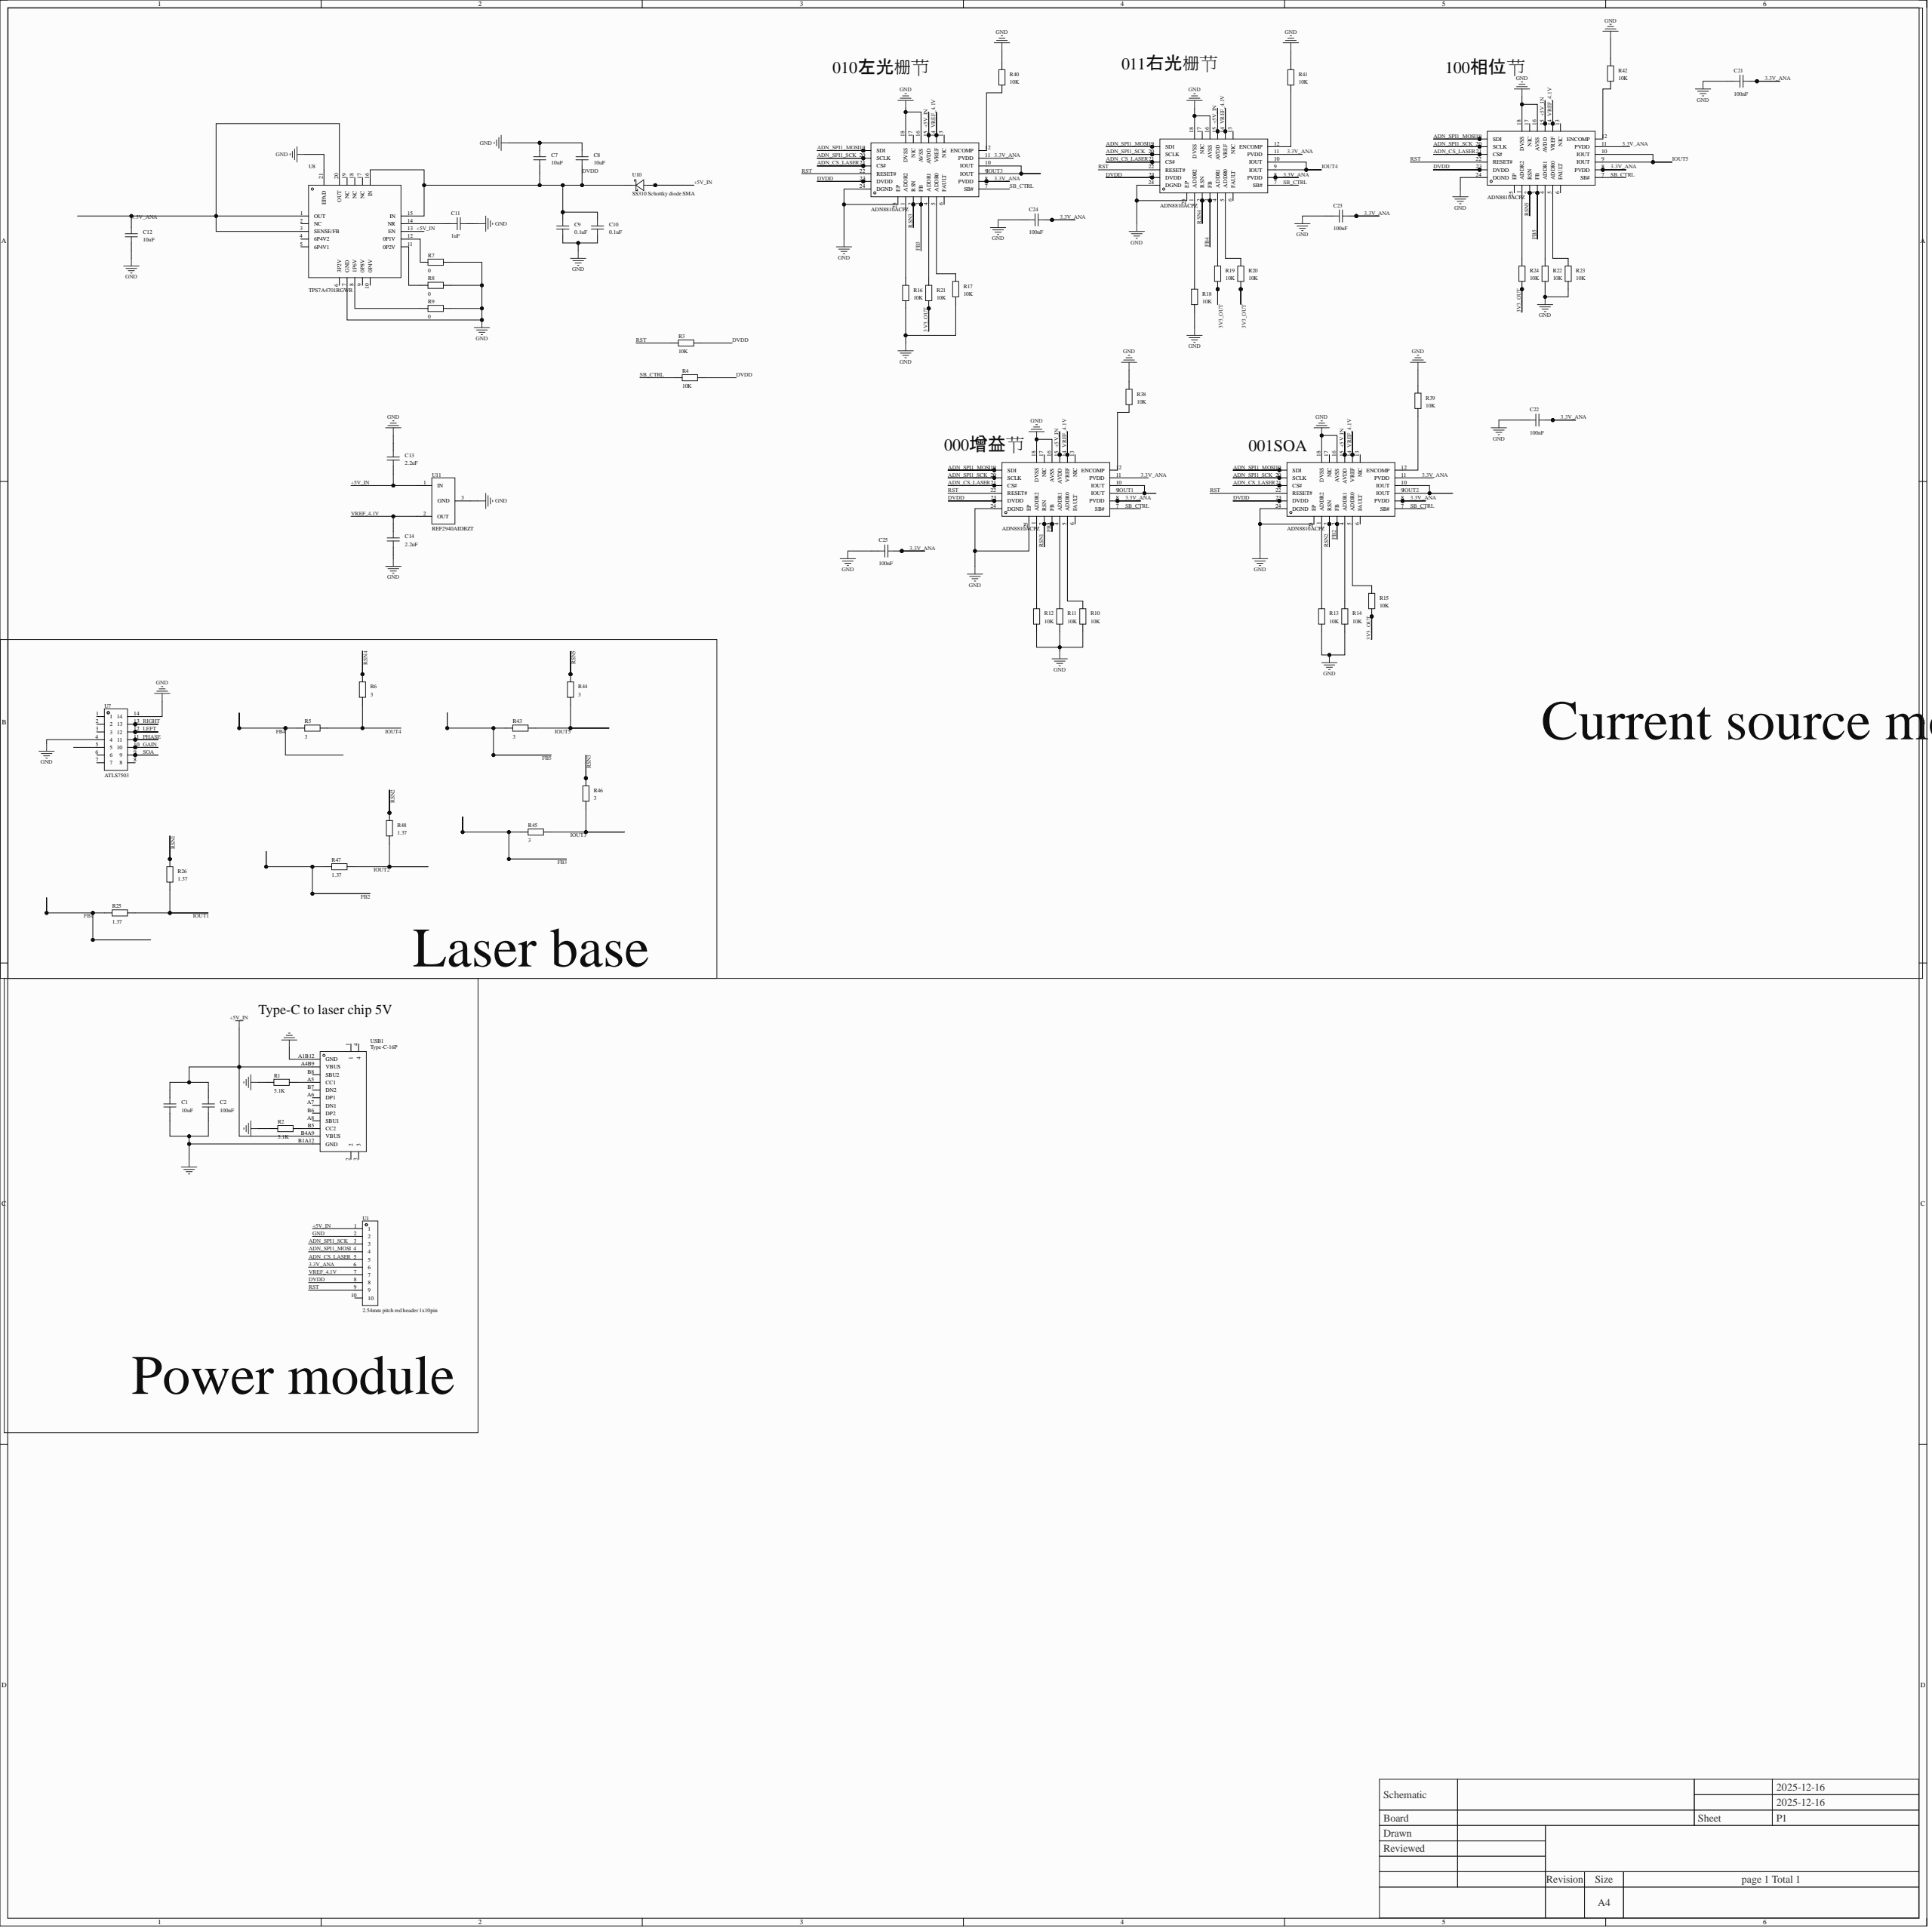Circuit board | Altium Designer | 63 parts | 52 nets
Bill of materials:
Comment,Description,Designator,Footprint,LibRef,Quantity
"ADN8810ACPZ","Output current: 300mA;","000增益节, 001SOA, 010左光栅节, 011右光栅节, 100相位节","LFCSP-24_L4.0-W4.0-P0.50-BL-EP2.3","ADN8810ACPZ","5"
"10uF","Capacitance: 10nF; accuracy: ±10%; rated voltage: 16V; temperature coefficient: X7R;","C1","C0402","AC0402KRX7R7BB103","1"
"100nF","Capacitance: 10nF; accuracy: ±10%; rated voltage: 16V; temperature coefficient: X7R;","C2","C0402","AC0402KRX7R7BB103","1"
"10uF","","C7, C8, C12","C0603","CAP_0603","3"
"0.1uF","","C9, C10","C0603","CAP_0603","2"
"1uF","","C11","C0603","CAP_0603","1"
"2.2uF","","C13, C14","C0603","CAP_0603","2"
"100nF","","C21, C22, C23, C24, C25","C0603","CAP_0603","5"
"5.1K","","R1, R2","R0603","Res_0603","2"
"10K","","R3, R4, R10, R11, R12, R13, R14, R15, R16, R17, R18, R19, R20, R21, R22, R23, R24, R38, R39, R40, R41, R42","R0603","Res_0603","22"
"3","","R5, R6, R43, R44, R45, R46","R0603","Res_0603","6"
"0","","R7, R8, R9","R0603","Res_0603","3"
"1.37","","R25, R26, R47, R48","R0603","Res_0603","4"
"2.54mm pitch red header 1x10pin","","U1","HDR-TH_10P-P2.54-V-F-2","间距2.54mm红色排母座1x10pin","1"
"ATLS7503","","U7","HDR-SMD_14P-P1.27-V-F-R2-C7-LS4.8","HEADER7X2B","1"
"TPS7A4701RGWR","Output type: adjustable; working voltage: 35V; output voltage: 1.4V~34V; output current: 1A; power supply rejection ratio (PSRR): 78dB@(1kHz); output polarity: positive;","U8","VQFN-20_L5.0-W5.0-P0.65-TL-EP","TPS7A4701RGWR","1"
"SS310 Schottky diode SMA","","U10","SMA_L4.3-W2.6-LS5.1-R-RD","SS310肖特基二极管SMA","1"
"REF2940AIDBZT","Output type: fixed; input voltage: 4.146V~5.5V; output voltage: 4.096V; output current: 25mA; accuracy: ±2%;","U11","SOT-23-3_L2.9-W1.3-P1.90-LS2.4-BR","REF2940AIDBZT","1"
"Type-C-16P","","USB1","USB-C-SMD_GT-USB-7010E","Type-C-16P","1"
Netlist (Protel format):
[
000增益节
LFCSP-24_L4.0-W4.0-P0.50-BL-EP2.3
ADN8810ACPZ



]
[
001SOA
LFCSP-24_L4.0-W4.0-P0.50-BL-EP2.3
ADN8810ACPZ



]
[
010左光栅节
LFCSP-24_L4.0-W4.0-P0.50-BL-EP2.3
ADN8810ACPZ



]
[
011右光栅节
LFCSP-24_L4.0-W4.0-P0.50-BL-EP2.3
ADN8810ACPZ



]
[
100相位节
LFCSP-24_L4.0-W4.0-P0.50-BL-EP2.3
ADN8810ACPZ



]
[
C1
C0402
10uF



]
[
C2
C0402
100nF



]
[
C7
C0603
10uF



]
[
C8
C0603
10uF



]
[
C9
C0603
0.1uF



]
[
C10
C0603
0.1uF



]
[
C11
C0603
1uF



]
[
C12
C0603
10uF



]
[
C13
C0603
2.2uF



]
[
C14
C0603
2.2uF



]
[
C21
C0603
100nF



]
[
C22
C0603
100nF



]
[
C23
C0603
100nF



]
[
C24
C0603
100nF



]
[
C25
C0603
100nF



]
[
R1
R0603
5.1K



]
[
R2
R0603
5.1K



]
[
R3
R0603
10K



]
[
R4
R0603
10K



]
[
R5
R0603
3



]
[
R6
R0603
3



]
[
R7
R0603
0



]
[
R8
R0603
0



]
[
R9
R0603
0



]
[
R10
R0603
10K



]
[
R11
R0603
10K



]
[
R12
R0603
10K



]
[
R13
R0603
10K



]
[
R14
R0603
10K



]
[
R15
R0603
10K



]
[
R16
R0603
10K



]
[
R17
R0603
10K



]
[
R18
R0603
10K



]
[
R19
R0603
10K



]
[
R20
R0603
10K



]
[
R21
R0603
10K



]
[
R22
R0603
10K



]
[
R23
R0603
10K



]
[
R24
R0603
10K



]
[
R25
R0603
1.37



]
[
R26
R0603
1.37



]
[
R38
R0603
10K



]
[
R39
R0603
10K



]
[
R40
R0603
10K



]
[
R41
R0603
10K



]
[
R42
R0603
10K



]
[
R43
R0603
3



]
[
R44
R0603
3



]
[
R45
R0603
3



]
[
R46
R0603
3



]
[
R47
R0603
1.37



]
[
R48
R0603
1.37



]
[
U1
HDR-TH_10P-P2.54-V-F-2
2.54mm pitch red header 1x10pin



]
[
U7
HDR-SMD_14P-P1.27-V-F-R2-C7-LS4.8
ATLS7503



]
[
U8
VQFN-20_L5.0-W5.0-P0.65-TL-EP
TPS7A4701RGWR



]
[
U10
SMA_L4.3-W2.6-LS5.1-R-RD
SS310 Schottky diode SMA



]
[
U11
SOT-23-3_L2.9-W1.3-P1.90-LS2.4-BR
REF2940AIDBZT



]
[
USB1
USB-C-SMD_GT-USB-7010E
Type-C-16P



]
(
VREF_4.1V
000增益节-14
001SOA-14
010左光栅节-14
011右光栅节-14
100相位节-14
C14-2
U1-7
U11-2
)
(
SB_CTRL
000增益节-7
001SOA-7
010左光栅节-7
011右光栅节-7
100相位节-7
R4-1
)
(
RST
000增益节-22
001SOA-22
010左光栅节-22
011右光栅节-22
100相位节-22
R3-1
U1-9
)
(
RSN5
100相位节-2
R44-1
)
(
RSN4
011右光栅节-2
R6-1
)
(
RSN3
010左光栅节-2
R46-1
)
(
RSN2
001SOA-2
R48-1
)
(
RSN1
000增益节-2
R26-1
)
(
NetR9_1
R9-1
U8-8
)
(
NetR8_1
R8-1
U8-11
)
(
NetR7_1
R7-1
U8-12
)
(
NetR2_2
R2-2
USB1-B5
)
(
NetR1_2
R1-2
USB1-A5
)
(
NetC11_2
C11-2
U8-14
)
(
Net100相位节_12
100相位节-12
R42-1
)
(
Net100相位节_5
100相位节-5
R23-2
)
(
Net100相位节_4
100相位节-4
R22-2
)
(
Net100相位节_1
100相位节-1
R24-2
)
(
Net011右光栅节_12
011右光栅节-12
R41-1
)
(
Net011右光栅节_5
011右光栅节-5
R20-2
)
(
Net011右光栅节_4
011右光栅节-4
R19-2
)
(
Net011右光栅节_1
011右光栅节-1
R18-2
)
(
Net010左光栅节_12
010左光栅节-12
R40-1
)
(
Net010左光栅节_5
010左光栅节-5
R17-2
)
(
Net010左光栅节_4
010左光栅节-4
R21-2
)
(
Net010左光栅节_1
010左光栅节-1
R16-2
)
(
Net001SOA_12
001SOA-12
R39-1
)
(
Net001SOA_5
001SOA-5
R15-2
)
(
Net001SOA_4
001SOA-4
R14-2
)
(
Net001SOA_1
001SOA-1
R13-2
)
(
Net000增益节_12
000增益节-12
R38-1
)
(
Net000增益节_5
000增益节-5
R10-2
)
(
Net000增益节_4
000增益节-4
R11-2
)
(
Net000增益节_1
000增益节-1
R12-2
)
(
IOUT5
100相位节-9
100相位节-10
R43-1
R44-2
)
(
IOUT4
011右光栅节-9
011右光栅节-10
R5-1
R6-2
)
(
IOUT3
010左光栅节-9
010左光栅节-10
R45-1
R46-2
)
(
IOUT2
001SOA-9
001SOA-10
R47-1
R48-2
)
(
IOUT1
000增益节-9
000增益节-10
R25-1
R26-2
)
(
GND
000增益节-16
000增益节-18
000增益节-24
000增益节-25
001SOA-16
001SOA-18
001SOA-24
001SOA-25
010左光栅节-16
010左光栅节-18
010左光栅节-24
010左光栅节-25
011右光栅节-16
011右光栅节-18
011右光栅节-24
011右光栅节-25
100相位节-16
100相位节-18
100相位节-24
C1-1
C2-1
C7-2
C8-2
C9-1
C10-1
C11-1
C12-1
C13-2
C14-1
C21-2
C22-2
C23-2
C24-2
C25-2
R1-1
R2-1
R7-2
R8-2
R9-2
R10-1
R11-1
R12-1
R13-1
R14-1
R16-1
R17-1
R18-1
R22-1
R23-1
R38-2
R39-2
R40-2
R41-2
R42-2
U1-2
U7-4
U7-14
U8-7
U8-21
U11-3
USB1-A1B12
USB1-B1A12
)
(
FB5
100相位节-3
R43-2
U7-11
)
(
FB4
011右光栅节-3
R5-2
U7-13
)
(
FB3
010左光栅节-3
R45-2
U7-12
)
(
FB2
001SOA-3
R47-2
U7-9
)
(
FB1
000增益节-3
R25-2
U7-10
)
(
DVDD
000增益节-23
001SOA-23
010左光栅节-23
011右光栅节-23
100相位节-23
C7-1
C8-1
C9-2
C10-2
R3-2
R4-2
U1-8
U8-15
U8-16
U10-2
)
(
ADN_SPI1_SCK
000增益节-20
001SOA-20
010左光栅节-20
011右光栅节-20
100相位节-20
U1-3
)
(
ADN_SPI1_MOSI
000增益节-19
001SOA-19
010左光栅节-19
011右光栅节-19
100相位节-19
U1-4
)
(
ADN_CS_LASER
000增益节-21
001SOA-21
010左光栅节-21
011右光栅节-21
100相位节-21
U1-5
)
(
+5V_IN
000增益节-15
001SOA-15
010左光栅节-15
011右光栅节-15
100相位节-15
C1-2
C2-2
C13-1
U1-1
U8-13
U10-1
U11-1
USB1-A4B9
USB1-B4A9
)
(
3V3_OUT
R15-1
R19-1
R20-1
R21-1
R24-1
)
(
3.3V_ANA
000增益节-8
000增益节-11
001SOA-8
001SOA-11
010左光栅节-8
010左光栅节-11
011右光栅节-8
011右光栅节-11
100相位节-8
100相位节-11
C12-2
C21-1
C22-1
C23-1
C24-1
C25-1
U1-6
U8-1
U8-3
U8-20
)